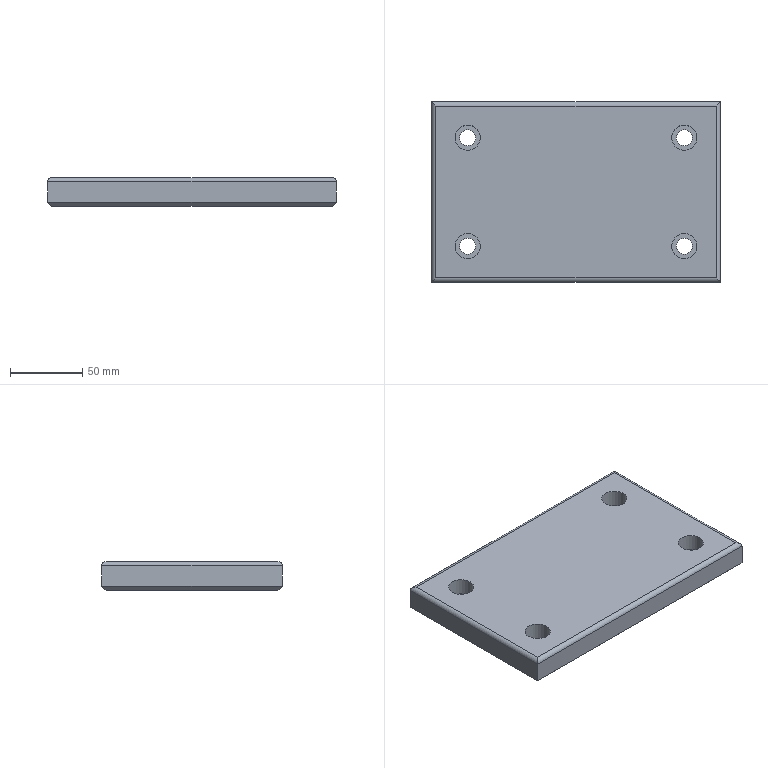Part | NX | features solid 2 | 1 solid | 26 faces | box 200 x 125 x 20 mm | volume 481280 mm3 | plane 14 | cylinder 12 | commonest cylinder face diameters 6 x4 11 x4 17.5 x4
STEP:
#1=CARTESIAN_POINT('',(495.,295.,-487.));
#2=VERTEX_POINT('',#1);
#3=CARTESIAN_POINT('',(495.,295.,-473.));
#4=VERTEX_POINT('',#3);
#5=CARTESIAN_POINT('',(495.,295.,-490.));
#6=DIRECTION('',(0.,0.,1.));
#7=VECTOR('',#6,1000.);
#8=LINE('',#5,#7);
#9=EDGE_CURVE('',#2,#4,#8,.T.);
#10=ORIENTED_EDGE('',*,*,#9,.T.);
#11=CARTESIAN_POINT('',(495.,420.,-473.));
#12=VERTEX_POINT('',#11);
#13=CARTESIAN_POINT('',(495.,295.,-473.));
#14=DIRECTION('',(0.,-1.,0.));
#15=VECTOR('',#14,1000.);
#16=LINE('',#13,#15);
#17=EDGE_CURVE('',#12,#4,#16,.T.);
#18=ORIENTED_EDGE('',*,*,#17,.F.);
#19=CARTESIAN_POINT('',(495.,420.,-487.));
#20=VERTEX_POINT('',#19);
#21=CARTESIAN_POINT('',(495.,420.,-490.));
#22=DIRECTION('',(0.,0.,1.));
#23=VECTOR('',#22,1000.);
#24=LINE('',#21,#23);
#25=EDGE_CURVE('',#20,#12,#24,.T.);
#26=ORIENTED_EDGE('',*,*,#25,.F.);
#27=CARTESIAN_POINT('',(495.,445.,-487.));
#28=DIRECTION('',(0.,1.,0.));
#29=VECTOR('',#28,1000.);
#30=LINE('',#27,#29);
#31=EDGE_CURVE('',#2,#20,#30,.T.);
#32=ORIENTED_EDGE('',*,*,#31,.F.);
#33=EDGE_LOOP('',(#10,#18,#26,#32));
#34=FACE_BOUND('',#33,.T.);
#35=CARTESIAN_POINT('',(495.,445.,-490.));
#36=DIRECTION('',(1.,0.,0.));
#37=DIRECTION('',(0.,1.,0.));
#38=AXIS2_PLACEMENT_3D('',#35,#36,#37);
#39=PLANE('',#38);
#40=ADVANCED_FACE('',(#34),#39,.F.);
#41=CARTESIAN_POINT('',(695.,295.,-487.));
#42=VERTEX_POINT('',#41);
#43=CARTESIAN_POINT('',(695.,295.,-473.));
#44=VERTEX_POINT('',#43);
#45=CARTESIAN_POINT('',(695.,295.,-490.));
#46=DIRECTION('',(0.,0.,1.));
#47=VECTOR('',#46,1000.);
#48=LINE('',#45,#47);
#49=EDGE_CURVE('',#42,#44,#48,.T.);
#50=ORIENTED_EDGE('',*,*,#49,.T.);
#51=CARTESIAN_POINT('',(695.,295.,-473.));
#52=DIRECTION('',(1.,0.,0.));
#53=VECTOR('',#52,1000.);
#54=LINE('',#51,#53);
#55=EDGE_CURVE('',#4,#44,#54,.T.);
#56=ORIENTED_EDGE('',*,*,#55,.F.);
#57=ORIENTED_EDGE('',*,*,#9,.F.);
#58=CARTESIAN_POINT('',(495.,295.,-487.));
#59=DIRECTION('',(-1.,0.,0.));
#60=VECTOR('',#59,1000.);
#61=LINE('',#58,#60);
#62=EDGE_CURVE('',#42,#2,#61,.T.);
#63=ORIENTED_EDGE('',*,*,#62,.F.);
#64=EDGE_LOOP('',(#50,#56,#57,#63));
#65=FACE_BOUND('',#64,.T.);
#66=CARTESIAN_POINT('',(495.,295.,-490.));
#67=DIRECTION('',(0.,1.,0.));
#68=DIRECTION('',(0.,0.,-1.));
#69=AXIS2_PLACEMENT_3D('',#66,#67,#68);
#70=PLANE('',#69);
#71=ADVANCED_FACE('',(#65),#70,.F.);
#72=CARTESIAN_POINT('',(695.,420.,-487.));
#73=VERTEX_POINT('',#72);
#74=CARTESIAN_POINT('',(695.,420.,-473.));
#75=VERTEX_POINT('',#74);
#76=CARTESIAN_POINT('',(695.,420.,-490.));
#77=DIRECTION('',(0.,0.,1.));
#78=VECTOR('',#77,1000.);
#79=LINE('',#76,#78);
#80=EDGE_CURVE('',#73,#75,#79,.T.);
#81=ORIENTED_EDGE('',*,*,#80,.T.);
#82=CARTESIAN_POINT('',(695.,445.,-473.));
#83=DIRECTION('',(0.,1.,0.));
#84=VECTOR('',#83,1000.);
#85=LINE('',#82,#84);
#86=EDGE_CURVE('',#44,#75,#85,.T.);
#87=ORIENTED_EDGE('',*,*,#86,.F.);
#88=ORIENTED_EDGE('',*,*,#49,.F.);
#89=CARTESIAN_POINT('',(695.,295.,-487.));
#90=DIRECTION('',(0.,-1.,0.));
#91=VECTOR('',#90,1000.);
#92=LINE('',#89,#91);
#93=EDGE_CURVE('',#73,#42,#92,.T.);
#94=ORIENTED_EDGE('',*,*,#93,.F.);
#95=EDGE_LOOP('',(#81,#87,#88,#94));
#96=FACE_BOUND('',#95,.T.);
#97=CARTESIAN_POINT('',(695.,295.,-490.));
#98=DIRECTION('',(-1.,0.,0.));
#99=DIRECTION('',(0.,0.,-1.));
#100=AXIS2_PLACEMENT_3D('',#97,#98,#99);
#101=PLANE('',#100);
#102=ADVANCED_FACE('',(#96),#101,.F.);
#103=ORIENTED_EDGE('',*,*,#25,.T.);
#104=CARTESIAN_POINT('',(495.,420.,-473.));
#105=DIRECTION('',(-1.,0.,0.));
#106=VECTOR('',#105,1000.);
#107=LINE('',#104,#106);
#108=EDGE_CURVE('',#75,#12,#107,.T.);
#109=ORIENTED_EDGE('',*,*,#108,.F.);
#110=ORIENTED_EDGE('',*,*,#80,.F.);
#111=CARTESIAN_POINT('',(695.,420.,-487.));
#112=DIRECTION('',(1.,0.,0.));
#113=VECTOR('',#112,1000.);
#114=LINE('',#111,#113);
#115=EDGE_CURVE('',#20,#73,#114,.T.);
#116=ORIENTED_EDGE('',*,*,#115,.F.);
#117=EDGE_LOOP('',(#103,#109,#110,#116));
#118=FACE_BOUND('',#117,.T.);
#119=CARTESIAN_POINT('',(695.,420.,-490.));
#120=DIRECTION('',(0.,-1.,0.));
#121=DIRECTION('',(1.,0.,0.));
#122=AXIS2_PLACEMENT_3D('',#119,#120,#121);
#123=PLANE('',#122);
#124=ADVANCED_FACE('',(#118),#123,.F.);
#125=CARTESIAN_POINT('',(498.,298.,-490.));
#126=VERTEX_POINT('',#125);
#127=CARTESIAN_POINT('',(692.,298.,-490.));
#128=VERTEX_POINT('',#127);
#129=CARTESIAN_POINT('',(495.,298.,-490.));
#130=DIRECTION('',(1.,0.,0.));
#131=VECTOR('',#130,1000.);
#132=LINE('',#129,#131);
#133=EDGE_CURVE('',#126,#128,#132,.T.);
#134=ORIENTED_EDGE('',*,*,#133,.F.);
#135=CARTESIAN_POINT('',(498.,417.,-490.));
#136=VERTEX_POINT('',#135);
#137=CARTESIAN_POINT('',(498.,445.,-490.));
#138=DIRECTION('',(0.,-1.,0.));
#139=VECTOR('',#138,1000.);
#140=LINE('',#137,#139);
#141=EDGE_CURVE('',#136,#126,#140,.T.);
#142=ORIENTED_EDGE('',*,*,#141,.F.);
#143=CARTESIAN_POINT('',(692.,417.,-490.));
#144=VERTEX_POINT('',#143);
#145=CARTESIAN_POINT('',(495.,417.,-490.));
#146=DIRECTION('',(-1.,0.,0.));
#147=VECTOR('',#146,1000.);
#148=LINE('',#145,#147);
#149=EDGE_CURVE('',#144,#136,#148,.T.);
#150=ORIENTED_EDGE('',*,*,#149,.F.);
#151=CARTESIAN_POINT('',(692.,445.,-490.));
#152=DIRECTION('',(0.,1.,0.));
#153=VECTOR('',#152,1000.);
#154=LINE('',#151,#153);
#155=EDGE_CURVE('',#128,#144,#154,.T.);
#156=ORIENTED_EDGE('',*,*,#155,.F.);
#157=EDGE_LOOP('',(#134,#142,#150,#156));
#158=FACE_BOUND('',#157,.T.);
#159=CARTESIAN_POINT('',(664.5,320.,-490.));
#160=VERTEX_POINT('',#159);
#161=CARTESIAN_POINT('',(670.,320.,-490.));
#162=DIRECTION('',(0.,0.,-1.));
#163=DIRECTION('',(-1.,0.,0.));
#164=AXIS2_PLACEMENT_3D('',#161,#162,#163);
#165=CIRCLE('',#164,5.5);
#166=EDGE_CURVE('',#160,#160,#165,.T.);
#167=ORIENTED_EDGE('',*,*,#166,.F.);
#168=EDGE_LOOP('',(#167));
#169=FACE_BOUND('',#168,.T.);
#170=CARTESIAN_POINT('',(664.5,395.,-490.));
#171=VERTEX_POINT('',#170);
#172=CARTESIAN_POINT('',(670.,395.,-490.));
#173=DIRECTION('',(0.,0.,-1.));
#174=DIRECTION('',(-1.,0.,0.));
#175=AXIS2_PLACEMENT_3D('',#172,#173,#174);
#176=CIRCLE('',#175,5.5);
#177=EDGE_CURVE('',#171,#171,#176,.T.);
#178=ORIENTED_EDGE('',*,*,#177,.F.);
#179=EDGE_LOOP('',(#178));
#180=FACE_BOUND('',#179,.T.);
#181=CARTESIAN_POINT('',(514.5,320.,-490.));
#182=VERTEX_POINT('',#181);
#183=CARTESIAN_POINT('',(520.,320.,-490.));
#184=DIRECTION('',(0.,0.,-1.));
#185=DIRECTION('',(-1.,0.,0.));
#186=AXIS2_PLACEMENT_3D('',#183,#184,#185);
#187=CIRCLE('',#186,5.5);
#188=EDGE_CURVE('',#182,#182,#187,.T.);
#189=ORIENTED_EDGE('',*,*,#188,.F.);
#190=EDGE_LOOP('',(#189));
#191=FACE_BOUND('',#190,.T.);
#192=CARTESIAN_POINT('',(514.5,395.,-490.));
#193=VERTEX_POINT('',#192);
#194=CARTESIAN_POINT('',(520.,395.,-490.));
#195=DIRECTION('',(0.,0.,-1.));
#196=DIRECTION('',(-1.,0.,0.));
#197=AXIS2_PLACEMENT_3D('',#194,#195,#196);
#198=CIRCLE('',#197,5.5);
#199=EDGE_CURVE('',#193,#193,#198,.T.);
#200=ORIENTED_EDGE('',*,*,#199,.F.);
#201=EDGE_LOOP('',(#200));
#202=FACE_BOUND('',#201,.T.);
#203=CARTESIAN_POINT('',(495.,445.,-490.));
#204=DIRECTION('',(0.,0.,1.));
#205=DIRECTION('',(-1.,0.,0.));
#206=AXIS2_PLACEMENT_3D('',#203,#204,#205);
#207=PLANE('',#206);
#208=ADVANCED_FACE('',(#158,#169,#180,#191,#202),#207,.F.);
#209=CARTESIAN_POINT('',(498.,298.,-470.));
#210=VERTEX_POINT('',#209);
#211=CARTESIAN_POINT('',(498.,417.,-470.));
#212=VERTEX_POINT('',#211);
#213=CARTESIAN_POINT('',(498.,445.,-470.));
#214=DIRECTION('',(0.,-1.,0.));
#215=VECTOR('',#214,1000.);
#216=LINE('',#213,#215);
#217=EDGE_CURVE('',#210,#212,#216,.F.);
#218=ORIENTED_EDGE('',*,*,#217,.F.);
#219=CARTESIAN_POINT('',(692.,298.,-470.));
#220=VERTEX_POINT('',#219);
#221=CARTESIAN_POINT('',(495.,298.,-470.));
#222=DIRECTION('',(1.,0.,0.));
#223=VECTOR('',#222,1000.);
#224=LINE('',#221,#223);
#225=EDGE_CURVE('',#220,#210,#224,.F.);
#226=ORIENTED_EDGE('',*,*,#225,.F.);
#227=CARTESIAN_POINT('',(692.,417.,-470.));
#228=VERTEX_POINT('',#227);
#229=CARTESIAN_POINT('',(692.,295.,-470.));
#230=DIRECTION('',(0.,1.,0.));
#231=VECTOR('',#230,1000.);
#232=LINE('',#229,#231);
#233=EDGE_CURVE('',#228,#220,#232,.F.);
#234=ORIENTED_EDGE('',*,*,#233,.F.);
#235=CARTESIAN_POINT('',(695.,417.,-470.));
#236=DIRECTION('',(-1.,0.,0.));
#237=VECTOR('',#236,1000.);
#238=LINE('',#235,#237);
#239=EDGE_CURVE('',#212,#228,#238,.F.);
#240=ORIENTED_EDGE('',*,*,#239,.F.);
#241=EDGE_LOOP('',(#218,#226,#234,#240));
#242=FACE_BOUND('',#241,.T.);
#243=CARTESIAN_POINT('',(678.75,320.,-470.));
#244=VERTEX_POINT('',#243);
#245=CARTESIAN_POINT('',(670.,320.,-470.));
#246=DIRECTION('',(0.,0.,1.));
#247=DIRECTION('',(1.,0.,0.));
#248=AXIS2_PLACEMENT_3D('',#245,#246,#247);
#249=CIRCLE('',#248,8.75);
#250=EDGE_CURVE('',#244,#244,#249,.T.);
#251=ORIENTED_EDGE('',*,*,#250,.F.);
#252=EDGE_LOOP('',(#251));
#253=FACE_BOUND('',#252,.T.);
#254=CARTESIAN_POINT('',(678.75,395.,-470.));
#255=VERTEX_POINT('',#254);
#256=CARTESIAN_POINT('',(670.,395.,-470.));
#257=DIRECTION('',(0.,0.,1.));
#258=DIRECTION('',(1.,0.,0.));
#259=AXIS2_PLACEMENT_3D('',#256,#257,#258);
#260=CIRCLE('',#259,8.75);
#261=EDGE_CURVE('',#255,#255,#260,.T.);
#262=ORIENTED_EDGE('',*,*,#261,.F.);
#263=EDGE_LOOP('',(#262));
#264=FACE_BOUND('',#263,.T.);
#265=CARTESIAN_POINT('',(528.75,320.,-470.));
#266=VERTEX_POINT('',#265);
#267=CARTESIAN_POINT('',(520.,320.,-470.));
#268=DIRECTION('',(0.,0.,1.));
#269=DIRECTION('',(1.,0.,0.));
#270=AXIS2_PLACEMENT_3D('',#267,#268,#269);
#271=CIRCLE('',#270,8.75);
#272=EDGE_CURVE('',#266,#266,#271,.T.);
#273=ORIENTED_EDGE('',*,*,#272,.F.);
#274=EDGE_LOOP('',(#273));
#275=FACE_BOUND('',#274,.T.);
#276=CARTESIAN_POINT('',(528.75,395.,-470.));
#277=VERTEX_POINT('',#276);
#278=CARTESIAN_POINT('',(520.,395.,-470.));
#279=DIRECTION('',(0.,0.,1.));
#280=DIRECTION('',(1.,0.,0.));
#281=AXIS2_PLACEMENT_3D('',#278,#279,#280);
#282=CIRCLE('',#281,8.75);
#283=EDGE_CURVE('',#277,#277,#282,.T.);
#284=ORIENTED_EDGE('',*,*,#283,.F.);
#285=EDGE_LOOP('',(#284));
#286=FACE_BOUND('',#285,.T.);
#287=CARTESIAN_POINT('',(495.,445.,-470.));
#288=DIRECTION('',(0.,0.,1.));
#289=DIRECTION('',(-1.,0.,0.));
#290=AXIS2_PLACEMENT_3D('',#287,#288,#289);
#291=PLANE('',#290);
#292=ADVANCED_FACE('',(#242,#253,#264,#275,#286),#291,.T.);
#293=CARTESIAN_POINT('',(525.5,395.,-482.));
#294=VERTEX_POINT('',#293);
#295=CARTESIAN_POINT('',(520.,395.,-482.));
#296=DIRECTION('',(0.,0.,1.));
#297=DIRECTION('',(1.,0.,0.));
#298=AXIS2_PLACEMENT_3D('',#295,#296,#297);
#299=CIRCLE('',#298,5.5);
#300=EDGE_CURVE('',#294,#294,#299,.T.);
#301=ORIENTED_EDGE('',*,*,#300,.T.);
#302=EDGE_LOOP('',(#301));
#303=FACE_BOUND('',#302,.T.);
#304=ORIENTED_EDGE('',*,*,#199,.T.);
#305=EDGE_LOOP('',(#304));
#306=FACE_BOUND('',#305,.T.);
#307=CARTESIAN_POINT('',(520.,395.,-520.));
#308=DIRECTION('',(0.,0.,-1.));
#309=DIRECTION('',(1.,0.,0.));
#310=AXIS2_PLACEMENT_3D('',#307,#308,#309);
#311=CYLINDRICAL_SURFACE('',#310,5.5);
#312=ADVANCED_FACE('',(#303,#306),#311,.F.);
#313=ORIENTED_EDGE('',*,*,#300,.F.);
#314=EDGE_LOOP('',(#313));
#315=FACE_BOUND('',#314,.T.);
#316=CARTESIAN_POINT('',(528.75,395.,-482.));
#317=VERTEX_POINT('',#316);
#318=CARTESIAN_POINT('',(520.,395.,-482.));
#319=DIRECTION('',(0.,0.,1.));
#320=DIRECTION('',(1.,0.,0.));
#321=AXIS2_PLACEMENT_3D('',#318,#319,#320);
#322=CIRCLE('',#321,8.75);
#323=EDGE_CURVE('',#317,#317,#322,.T.);
#324=ORIENTED_EDGE('',*,*,#323,.T.);
#325=EDGE_LOOP('',(#324));
#326=FACE_BOUND('',#325,.T.);
#327=CARTESIAN_POINT('',(520.,395.,-482.));
#328=DIRECTION('',(0.,0.,-1.));
#329=DIRECTION('',(1.,0.,0.));
#330=AXIS2_PLACEMENT_3D('',#327,#328,#329);
#331=PLANE('',#330);
#332=ADVANCED_FACE('',(#315,#326),#331,.F.);
#333=ORIENTED_EDGE('',*,*,#323,.F.);
#334=EDGE_LOOP('',(#333));
#335=FACE_BOUND('',#334,.T.);
#336=ORIENTED_EDGE('',*,*,#283,.T.);
#337=EDGE_LOOP('',(#336));
#338=FACE_BOUND('',#337,.T.);
#339=CARTESIAN_POINT('',(520.,395.,-470.));
#340=DIRECTION('',(0.,0.,-1.));
#341=DIRECTION('',(1.,0.,0.));
#342=AXIS2_PLACEMENT_3D('',#339,#340,#341);
#343=CYLINDRICAL_SURFACE('',#342,8.75);
#344=ADVANCED_FACE('',(#335,#338),#343,.F.);
#345=CARTESIAN_POINT('',(525.5,320.,-482.));
#346=VERTEX_POINT('',#345);
#347=CARTESIAN_POINT('',(520.,320.,-482.));
#348=DIRECTION('',(0.,0.,1.));
#349=DIRECTION('',(1.,0.,0.));
#350=AXIS2_PLACEMENT_3D('',#347,#348,#349);
#351=CIRCLE('',#350,5.5);
#352=EDGE_CURVE('',#346,#346,#351,.T.);
#353=ORIENTED_EDGE('',*,*,#352,.T.);
#354=EDGE_LOOP('',(#353));
#355=FACE_BOUND('',#354,.T.);
#356=ORIENTED_EDGE('',*,*,#188,.T.);
#357=EDGE_LOOP('',(#356));
#358=FACE_BOUND('',#357,.T.);
#359=CARTESIAN_POINT('',(520.,320.,-520.));
#360=DIRECTION('',(0.,0.,-1.));
#361=DIRECTION('',(1.,0.,0.));
#362=AXIS2_PLACEMENT_3D('',#359,#360,#361);
#363=CYLINDRICAL_SURFACE('',#362,5.5);
#364=ADVANCED_FACE('',(#355,#358),#363,.F.);
#365=ORIENTED_EDGE('',*,*,#352,.F.);
#366=EDGE_LOOP('',(#365));
#367=FACE_BOUND('',#366,.T.);
#368=CARTESIAN_POINT('',(528.75,320.,-482.));
#369=VERTEX_POINT('',#368);
#370=CARTESIAN_POINT('',(520.,320.,-482.));
#371=DIRECTION('',(0.,0.,1.));
#372=DIRECTION('',(1.,0.,0.));
#373=AXIS2_PLACEMENT_3D('',#370,#371,#372);
#374=CIRCLE('',#373,8.75);
#375=EDGE_CURVE('',#369,#369,#374,.T.);
#376=ORIENTED_EDGE('',*,*,#375,.T.);
#377=EDGE_LOOP('',(#376));
#378=FACE_BOUND('',#377,.T.);
#379=CARTESIAN_POINT('',(520.,320.,-482.));
#380=DIRECTION('',(0.,0.,-1.));
#381=DIRECTION('',(1.,0.,0.));
#382=AXIS2_PLACEMENT_3D('',#379,#380,#381);
#383=PLANE('',#382);
#384=ADVANCED_FACE('',(#367,#378),#383,.F.);
#385=ORIENTED_EDGE('',*,*,#375,.F.);
#386=EDGE_LOOP('',(#385));
#387=FACE_BOUND('',#386,.T.);
#388=ORIENTED_EDGE('',*,*,#272,.T.);
#389=EDGE_LOOP('',(#388));
#390=FACE_BOUND('',#389,.T.);
#391=CARTESIAN_POINT('',(520.,320.,-470.));
#392=DIRECTION('',(0.,0.,-1.));
#393=DIRECTION('',(1.,0.,0.));
#394=AXIS2_PLACEMENT_3D('',#391,#392,#393);
#395=CYLINDRICAL_SURFACE('',#394,8.75);
#396=ADVANCED_FACE('',(#387,#390),#395,.F.);
#397=CARTESIAN_POINT('',(675.5,395.,-482.));
#398=VERTEX_POINT('',#397);
#399=CARTESIAN_POINT('',(670.,395.,-482.));
#400=DIRECTION('',(0.,0.,1.));
#401=DIRECTION('',(1.,0.,0.));
#402=AXIS2_PLACEMENT_3D('',#399,#400,#401);
#403=CIRCLE('',#402,5.5);
#404=EDGE_CURVE('',#398,#398,#403,.T.);
#405=ORIENTED_EDGE('',*,*,#404,.T.);
#406=EDGE_LOOP('',(#405));
#407=FACE_BOUND('',#406,.T.);
#408=ORIENTED_EDGE('',*,*,#177,.T.);
#409=EDGE_LOOP('',(#408));
#410=FACE_BOUND('',#409,.T.);
#411=CARTESIAN_POINT('',(670.,395.,-520.));
#412=DIRECTION('',(0.,0.,-1.));
#413=DIRECTION('',(1.,0.,0.));
#414=AXIS2_PLACEMENT_3D('',#411,#412,#413);
#415=CYLINDRICAL_SURFACE('',#414,5.5);
#416=ADVANCED_FACE('',(#407,#410),#415,.F.);
#417=ORIENTED_EDGE('',*,*,#404,.F.);
#418=EDGE_LOOP('',(#417));
#419=FACE_BOUND('',#418,.T.);
#420=CARTESIAN_POINT('',(678.75,395.,-482.));
#421=VERTEX_POINT('',#420);
#422=CARTESIAN_POINT('',(670.,395.,-482.));
#423=DIRECTION('',(0.,0.,1.));
#424=DIRECTION('',(1.,0.,0.));
#425=AXIS2_PLACEMENT_3D('',#422,#423,#424);
#426=CIRCLE('',#425,8.75);
#427=EDGE_CURVE('',#421,#421,#426,.T.);
#428=ORIENTED_EDGE('',*,*,#427,.T.);
#429=EDGE_LOOP('',(#428));
#430=FACE_BOUND('',#429,.T.);
#431=CARTESIAN_POINT('',(670.,395.,-482.));
#432=DIRECTION('',(0.,0.,-1.));
#433=DIRECTION('',(1.,0.,0.));
#434=AXIS2_PLACEMENT_3D('',#431,#432,#433);
#435=PLANE('',#434);
#436=ADVANCED_FACE('',(#419,#430),#435,.F.);
#437=ORIENTED_EDGE('',*,*,#427,.F.);
#438=EDGE_LOOP('',(#437));
#439=FACE_BOUND('',#438,.T.);
#440=ORIENTED_EDGE('',*,*,#261,.T.);
#441=EDGE_LOOP('',(#440));
#442=FACE_BOUND('',#441,.T.);
#443=CARTESIAN_POINT('',(670.,395.,-470.));
#444=DIRECTION('',(0.,0.,-1.));
#445=DIRECTION('',(1.,0.,0.));
#446=AXIS2_PLACEMENT_3D('',#443,#444,#445);
#447=CYLINDRICAL_SURFACE('',#446,8.75);
#448=ADVANCED_FACE('',(#439,#442),#447,.F.);
#449=CARTESIAN_POINT('',(675.5,320.,-482.));
#450=VERTEX_POINT('',#449);
#451=CARTESIAN_POINT('',(670.,320.,-482.));
#452=DIRECTION('',(0.,0.,1.));
#453=DIRECTION('',(1.,0.,0.));
#454=AXIS2_PLACEMENT_3D('',#451,#452,#453);
#455=CIRCLE('',#454,5.5);
#456=EDGE_CURVE('',#450,#450,#455,.T.);
#457=ORIENTED_EDGE('',*,*,#456,.T.);
#458=EDGE_LOOP('',(#457));
#459=FACE_BOUND('',#458,.T.);
#460=ORIENTED_EDGE('',*,*,#166,.T.);
#461=EDGE_LOOP('',(#460));
#462=FACE_BOUND('',#461,.T.);
#463=CARTESIAN_POINT('',(670.,320.,-520.));
#464=DIRECTION('',(0.,0.,-1.));
#465=DIRECTION('',(1.,0.,0.));
#466=AXIS2_PLACEMENT_3D('',#463,#464,#465);
#467=CYLINDRICAL_SURFACE('',#466,5.5);
#468=ADVANCED_FACE('',(#459,#462),#467,.F.);
#469=ORIENTED_EDGE('',*,*,#456,.F.);
#470=EDGE_LOOP('',(#469));
#471=FACE_BOUND('',#470,.T.);
#472=CARTESIAN_POINT('',(678.75,320.,-482.));
#473=VERTEX_POINT('',#472);
#474=CARTESIAN_POINT('',(670.,320.,-482.));
#475=DIRECTION('',(0.,0.,1.));
#476=DIRECTION('',(1.,0.,0.));
#477=AXIS2_PLACEMENT_3D('',#474,#475,#476);
#478=CIRCLE('',#477,8.75);
#479=EDGE_CURVE('',#473,#473,#478,.T.);
#480=ORIENTED_EDGE('',*,*,#479,.T.);
#481=EDGE_LOOP('',(#480));
#482=FACE_BOUND('',#481,.T.);
#483=CARTESIAN_POINT('',(670.,320.,-482.));
#484=DIRECTION('',(0.,0.,-1.));
#485=DIRECTION('',(1.,0.,0.));
#486=AXIS2_PLACEMENT_3D('',#483,#484,#485);
#487=PLANE('',#486);
#488=ADVANCED_FACE('',(#471,#482),#487,.F.);
#489=ORIENTED_EDGE('',*,*,#479,.F.);
#490=EDGE_LOOP('',(#489));
#491=FACE_BOUND('',#490,.T.);
#492=ORIENTED_EDGE('',*,*,#250,.T.);
#493=EDGE_LOOP('',(#492));
#494=FACE_BOUND('',#493,.T.);
#495=CARTESIAN_POINT('',(670.,320.,-470.));
#496=DIRECTION('',(0.,0.,-1.));
#497=DIRECTION('',(1.,0.,0.));
#498=AXIS2_PLACEMENT_3D('',#495,#496,#497);
#499=CYLINDRICAL_SURFACE('',#498,8.75);
#500=ADVANCED_FACE('',(#491,#494),#499,.F.);
#501=CARTESIAN_POINT('',(498.,298.,-473.));
#502=DIRECTION('',(0.7071,-0.7071,0.));
#503=DIRECTION('',(0.7071,0.7071,0.));
#504=AXIS2_PLACEMENT_3D('',#501,#502,#503);
#505=ELLIPSE('',#504,4.243,3.);
#506=EDGE_CURVE('',#210,#4,#505,.T.);
#507=ORIENTED_EDGE('',*,*,#506,.T.);
#508=ORIENTED_EDGE('',*,*,#55,.T.);
#509=CARTESIAN_POINT('',(692.,298.,-473.));
#510=DIRECTION('',(0.7071,0.7071,0.));
#511=DIRECTION('',(-0.7071,0.7071,0.));
#512=AXIS2_PLACEMENT_3D('',#509,#510,#511);
#513=ELLIPSE('',#512,4.243,3.);
#514=EDGE_CURVE('',#44,#220,#513,.F.);
#515=ORIENTED_EDGE('',*,*,#514,.T.);
#516=ORIENTED_EDGE('',*,*,#225,.T.);
#517=EDGE_LOOP('',(#507,#508,#515,#516));
#518=FACE_BOUND('',#517,.T.);
#519=CARTESIAN_POINT('',(495.,298.,-473.));
#520=DIRECTION('',(-1.,0.,0.));
#521=DIRECTION('',(0.,0.,-1.));
#522=AXIS2_PLACEMENT_3D('',#519,#520,#521);
#523=CYLINDRICAL_SURFACE('',#522,3.);
#524=ADVANCED_FACE('',(#518),#523,.T.);
#525=ORIENTED_EDGE('',*,*,#514,.F.);
#526=ORIENTED_EDGE('',*,*,#86,.T.);
#527=CARTESIAN_POINT('',(692.,417.,-473.));
#528=DIRECTION('',(-0.7071,0.7071,0.));
#529=DIRECTION('',(-0.7071,-0.7071,0.));
#530=AXIS2_PLACEMENT_3D('',#527,#528,#529);
#531=ELLIPSE('',#530,4.243,3.);
#532=EDGE_CURVE('',#75,#228,#531,.F.);
#533=ORIENTED_EDGE('',*,*,#532,.T.);
#534=ORIENTED_EDGE('',*,*,#233,.T.);
#535=EDGE_LOOP('',(#525,#526,#533,#534));
#536=FACE_BOUND('',#535,.T.);
#537=CARTESIAN_POINT('',(692.,295.,-473.));
#538=DIRECTION('',(0.,-1.,0.));
#539=DIRECTION('',(0.,0.,1.));
#540=AXIS2_PLACEMENT_3D('',#537,#538,#539);
#541=CYLINDRICAL_SURFACE('',#540,3.);
#542=ADVANCED_FACE('',(#536),#541,.T.);
#543=ORIENTED_EDGE('',*,*,#506,.F.);
#544=ORIENTED_EDGE('',*,*,#217,.T.);
#545=CARTESIAN_POINT('',(498.,417.,-473.));
#546=DIRECTION('',(-0.7071,-0.7071,0.));
#547=DIRECTION('',(-0.7071,0.7071,0.));
#548=AXIS2_PLACEMENT_3D('',#545,#546,#547);
#549=ELLIPSE('',#548,4.243,3.);
#550=EDGE_CURVE('',#212,#12,#549,.T.);
#551=ORIENTED_EDGE('',*,*,#550,.T.);
#552=ORIENTED_EDGE('',*,*,#17,.T.);
#553=EDGE_LOOP('',(#543,#544,#551,#552));
#554=FACE_BOUND('',#553,.T.);
#555=CARTESIAN_POINT('',(498.,445.,-473.));
#556=DIRECTION('',(0.,1.,0.));
#557=DIRECTION('',(-1.,0.,0.));
#558=AXIS2_PLACEMENT_3D('',#555,#556,#557);
#559=CYLINDRICAL_SURFACE('',#558,3.);
#560=ADVANCED_FACE('',(#554),#559,.T.);
#561=ORIENTED_EDGE('',*,*,#532,.F.);
#562=ORIENTED_EDGE('',*,*,#108,.T.);
#563=ORIENTED_EDGE('',*,*,#550,.F.);
#564=ORIENTED_EDGE('',*,*,#239,.T.);
#565=EDGE_LOOP('',(#561,#562,#563,#564));
#566=FACE_BOUND('',#565,.T.);
#567=CARTESIAN_POINT('',(695.,417.,-473.));
#568=DIRECTION('',(1.,0.,0.));
#569=DIRECTION('',(0.,1.,0.));
#570=AXIS2_PLACEMENT_3D('',#567,#568,#569);
#571=CYLINDRICAL_SURFACE('',#570,3.);
#572=ADVANCED_FACE('',(#566),#571,.T.);
#573=CARTESIAN_POINT('',(497.,418.,-489.));
#574=DIRECTION('',(0.5774,-0.5774,-0.5774));
#575=VECTOR('',#574,1000.);
#576=LINE('',#573,#575);
#577=EDGE_CURVE('',#20,#136,#576,.T.);
#578=ORIENTED_EDGE('',*,*,#577,.T.);
#579=ORIENTED_EDGE('',*,*,#141,.T.);
#580=CARTESIAN_POINT('',(547.,347.,-539.));
#581=DIRECTION('',(0.5774,0.5774,-0.5774));
#582=VECTOR('',#581,1000.);
#583=LINE('',#580,#582);
#584=EDGE_CURVE('',#126,#2,#583,.F.);
#585=ORIENTED_EDGE('',*,*,#584,.T.);
#586=ORIENTED_EDGE('',*,*,#31,.T.);
#587=EDGE_LOOP('',(#578,#579,#585,#586));
#588=FACE_BOUND('',#587,.T.);
#589=CARTESIAN_POINT('',(498.,445.,-490.));
#590=DIRECTION('',(0.7071,0.,0.7071));
#591=DIRECTION('',(-0.7071,0.,0.7071));
#592=AXIS2_PLACEMENT_3D('',#589,#590,#591);
#593=PLANE('',#592);
#594=ADVANCED_FACE('',(#588),#593,.F.);
#595=ORIENTED_EDGE('',*,*,#584,.F.);
#596=ORIENTED_EDGE('',*,*,#133,.T.);
#597=CARTESIAN_POINT('',(626.333,363.667,-555.667));
#598=DIRECTION('',(-0.5774,0.5774,-0.5774));
#599=VECTOR('',#598,1000.);
#600=LINE('',#597,#599);
#601=EDGE_CURVE('',#128,#42,#600,.F.);
#602=ORIENTED_EDGE('',*,*,#601,.T.);
#603=ORIENTED_EDGE('',*,*,#62,.T.);
#604=EDGE_LOOP('',(#595,#596,#602,#603));
#605=FACE_BOUND('',#604,.T.);
#606=CARTESIAN_POINT('',(495.,298.,-490.));
#607=DIRECTION('',(0.,0.7071,0.7071));
#608=DIRECTION('',(0.,0.7071,-0.7071));
#609=AXIS2_PLACEMENT_3D('',#606,#607,#608);
#610=PLANE('',#609);
#611=ADVANCED_FACE('',(#605),#610,.F.);
#612=ORIENTED_EDGE('',*,*,#577,.F.);
#613=ORIENTED_EDGE('',*,*,#115,.T.);
#614=CARTESIAN_POINT('',(626.333,351.333,-555.667));
#615=DIRECTION('',(0.5774,0.5774,0.5774));
#616=VECTOR('',#615,1000.);
#617=LINE('',#614,#616);
#618=EDGE_CURVE('',#73,#144,#617,.F.);
#619=ORIENTED_EDGE('',*,*,#618,.T.);
#620=ORIENTED_EDGE('',*,*,#149,.T.);
#621=EDGE_LOOP('',(#612,#613,#619,#620));
#622=FACE_BOUND('',#621,.T.);
#623=CARTESIAN_POINT('',(495.,417.,-490.));
#624=DIRECTION('',(0.,-0.7071,0.7071));
#625=DIRECTION('',(0.,0.7071,0.7071));
#626=AXIS2_PLACEMENT_3D('',#623,#624,#625);
#627=PLANE('',#626);
#628=ADVANCED_FACE('',(#622),#627,.F.);
#629=ORIENTED_EDGE('',*,*,#601,.F.);
#630=ORIENTED_EDGE('',*,*,#155,.T.);
#631=ORIENTED_EDGE('',*,*,#618,.F.);
#632=ORIENTED_EDGE('',*,*,#93,.T.);
#633=EDGE_LOOP('',(#629,#630,#631,#632));
#634=FACE_BOUND('',#633,.T.);
#635=CARTESIAN_POINT('',(692.,445.,-490.));
#636=DIRECTION('',(-0.7071,0.,0.7071));
#637=DIRECTION('',(-0.7071,0.,-0.7071));
#638=AXIS2_PLACEMENT_3D('',#635,#636,#637);
#639=PLANE('',#638);
#640=ADVANCED_FACE('',(#634),#639,.F.);
#641=CLOSED_SHELL('',(#40,#71,#102,#124,#208,#292,#312,#332,#344,#364,#384,#396,#416,#436,#448,#468,#488,#500,#524,#542,#560,#572,#594,#611,#628,#640));
#642=MANIFOLD_SOLID_BREP('',#641);
#643=(LENGTH_UNIT()NAMED_UNIT(*)SI_UNIT(.MILLI.,.METRE.));
#644=UNCERTAINTY_MEASURE_WITH_UNIT(LENGTH_MEASURE(0.00001),#643,'','');
#645=(NAMED_UNIT(*)PLANE_ANGLE_UNIT()SI_UNIT($,.RADIAN.));
#646=(NAMED_UNIT(*)SI_UNIT($,.STERADIAN.)SOLID_ANGLE_UNIT());
#647=(GEOMETRIC_REPRESENTATION_CONTEXT(3)GLOBAL_UNCERTAINTY_ASSIGNED_CONTEXT((#644))GLOBAL_UNIT_ASSIGNED_CONTEXT((#643,#645,#646))REPRESENTATION_CONTEXT('',''));
#648=ADVANCED_BREP_SHAPE_REPRESENTATION('',(#642),#647);